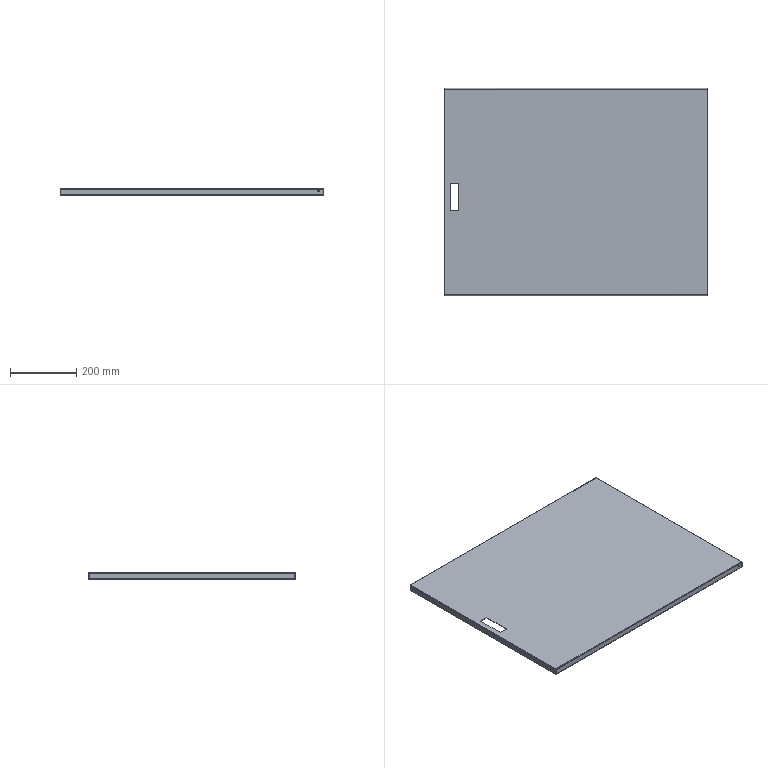Part | STEP file | 001-001-Machine frame door panel | 1 solid | 78 faces | box 795 x 624 x 20 mm | volume 869592 mm3 | plane 42 | cylinder 20 | spline 16 | commonest cylinder face diameters 1.473 x8 4.473 x8 6.5 x4